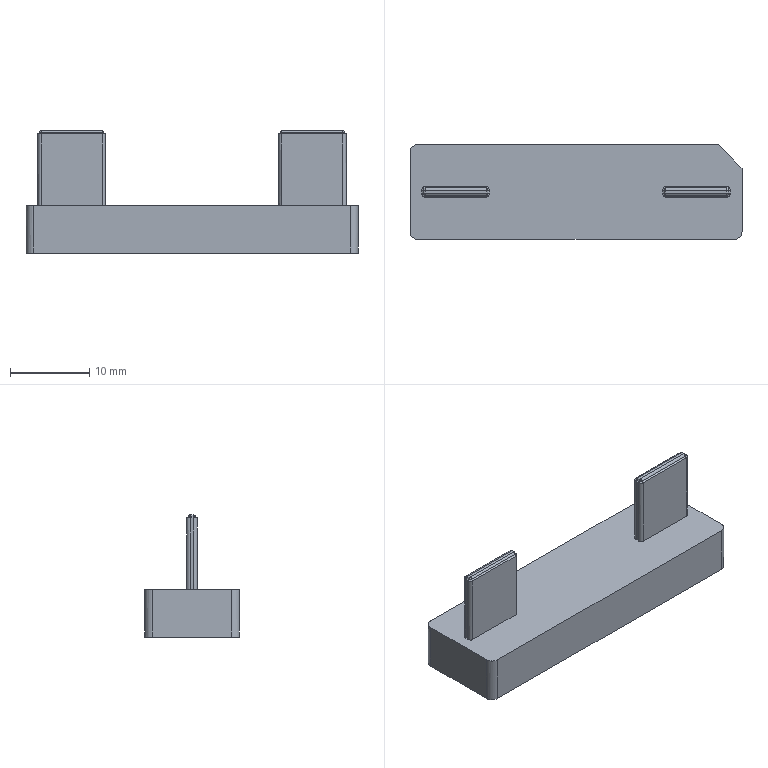NC program | PowerMill | posted with a generic post | part box 42 x 12 x 15.447 mm
Lines 5063 to 6058 of 88764:
N5160 M6
N5161 S18000 M03
N5162 G00 G90 X0.0 Y0.0
N5163 G43 Z9.7972 H2
N5164
N5165 G05 P10000 R4
N5166 X-16.8455 Y3.4637
N5167 Z0.7877
N5168 G01 Z-0.4123 F3600.0
N5169 X-16.8553 Y3.444 F6000.0
N5170 G03 X-16.7667 Y3.1783 I0.1771 J-0.0885
N5171 G01 X-15.3737 Y2.4822
N5172 X-11.7133 Y2.4829
N5173 X-11.2252 Y2.4763
N5174 X-10.7372 Y2.3846
N5175 X-10.2969 Y2.1962
N5176 X-9.7611 Y1.7673
N5177 X-9.3902 Y1.2201
N5178 X-9.2227 Y0.7321
N5179 X-9.1642 Y0.244
N5180 X-9.1662 Y-0.244
N5181 X-9.2316 Y-0.7321
N5182 X-9.4063 Y-1.2201
N5183 X-9.7365 Y-1.7082
N5184 X-10.2491 Y-2.1361
N5185 X-10.3552 Y-2.1962
N5186 X-10.7372 Y-2.3486
N5187 X-11.2252 Y-2.442
N5188 X-11.7133 Y-2.4487
N5189 X-19.0341 Y-2.4496
N5190 X-19.5221 Y-2.4047
N5191 X-20.0102 Y-2.2512
N5192 X-20.4982 Y-1.9437
N5193 X-20.7437 Y-1.7082
N5194 X-20.9863 Y-1.3814
N5195 X-21.0744 Y-1.2201
N5196 X-21.2494 Y-0.7321
N5197 X-21.3146 Y-0.244
N5198 X-21.3168 Y0.244
N5199 X-21.257 Y0.7321
N5200 X-21.0904 Y1.2201
N5201 X-20.9863 Y1.4141
N5202 X-20.7731 Y1.7082
N5203 X-20.4982 Y1.9737
N5204 X-20.184 Y2.1962
N5205 X-20.0102 Y2.2853
N5206 X-19.5221 Y2.4377
N5207 X-19.0341 Y2.4814
N5208 X-15.3737 Y2.4822
N5209 X-16.8055 Y3.6441 Z-0.6116
N5210 X-16.8154 Y3.6245
N5211 G03 X-16.7268 Y3.3588 I0.1771 J-0.0886
N5212 G01 X-15.3737 Y2.6822
N5213 X-11.7133
N5214 X-11.2252 Y2.6769
N5215 X-10.7372 Y2.5943
N5216 X-10.2491 Y2.3983
N5217 X-9.9368 Y2.1962
N5218 X-9.7611 Y2.0517
N5219 X-9.4529 Y1.7082
N5220 X-9.273 Y1.4244
N5221 X-9.1745 Y1.2201
N5222 X-9.0244 Y0.7321
N5223 X-8.9752 Y0.244
N5224 X-8.9755 Y-0.244
N5225 X-9.0306 Y-0.7321
N5226 X-9.1881 Y-1.2201
N5227 X-9.4766 Y-1.7082
N5228 X-9.7611 Y-2.0182
N5229 X-9.9783 Y-2.1962
N5230 X-10.2491 Y-2.3659
N5231 X-10.7372 Y-2.5618
N5232 X-11.2252 Y-2.6441
N5233 X-11.7133 Y-2.65
N5234 X-19.0341
N5235 X-19.5221 Y-2.6099
N5236 X-20.0102 Y-2.4692
N5237 X-20.4982 Y-2.1971
N5238 X-20.9863 Y-1.7303
N5239 X-21.2917 Y-1.2201
N5240 X-21.4492 Y-0.7321
N5241 X-21.5045 Y-0.244
N5242 X-21.5048 Y0.244
N5243 X-21.4743 Y0.6236
N5244 X-21.3056 Y1.2201
N5245 X-21.0273 Y1.7082
N5246 X-20.545 Y2.1962
N5247 X-20.0102 Y2.5013
N5248 X-19.5221 Y2.6441
N5249 X-19.0341 Y2.6822
N5250 X-15.3737
N5251 X-16.8055 Y3.6441 Z-0.8109
N5252 X-16.8154 Y3.6245
N5253 G03 X-16.7268 Y3.3588 I0.1771 J-0.0886
N5254 G01 X-15.3737 Y2.6822
N5255 X-11.7133
N5256 X-11.2252 Y2.6769
N5257 X-10.7372 Y2.5943
N5258 X-10.2491 Y2.3983
N5259 X-9.9368 Y2.1962
N5260 X-9.7611 Y2.0517
N5261 X-9.4529 Y1.7082
N5262 X-9.273 Y1.4244
N5263 X-9.1745 Y1.2201
N5264 X-9.0244 Y0.7321
N5265 X-8.9752 Y0.244
N5266 X-8.9755 Y-0.244
N5267 X-9.0306 Y-0.7321
N5268 X-9.1881 Y-1.2201
N5269 X-9.4766 Y-1.7082
N5270 X-9.7611 Y-2.0182
N5271 X-9.9783 Y-2.1962
N5272 X-10.2491 Y-2.3659
N5273 X-10.7372 Y-2.5618
N5274 X-11.2252 Y-2.6441
N5275 X-11.7133 Y-2.65
N5276 X-19.0341
N5277 X-19.5221 Y-2.6099
N5278 X-20.0102 Y-2.4692
N5279 X-20.4982 Y-2.1971
N5280 X-20.9863 Y-1.7303
N5281 X-21.2917 Y-1.2201
N5282 X-21.4492 Y-0.7321
N5283 X-21.5045 Y-0.244
N5284 X-21.5048 Y0.244
N5285 X-21.4743 Y0.6236
N5286 X-21.3056 Y1.2201
N5287 X-21.0273 Y1.7082
N5288 X-20.545 Y2.1962
N5289 X-20.0102 Y2.5013
N5290 X-19.5221 Y2.6441
N5291 X-19.0341 Y2.6822
N5292 X-15.3737
N5293 X-16.8055 Y3.6441 Z-1.0102
N5294 X-16.8154 Y3.6245
N5295 G03 X-16.7268 Y3.3588 I0.1771 J-0.0886
N5296 G01 X-15.3737 Y2.6822
N5297 X-11.7133
N5298 X-11.2252 Y2.6769
N5299 X-10.7372 Y2.5943
N5300 X-10.2491 Y2.3983
N5301 X-9.9368 Y2.1962
N5302 X-9.7611 Y2.0517
N5303 X-9.4529 Y1.7082
N5304 X-9.273 Y1.4245
N5305 X-9.1745 Y1.2201
N5306 X-9.0244 Y0.7321
N5307 X-8.9752 Y0.244
N5308 X-8.9755 Y-0.244
N5309 X-9.0306 Y-0.7321
N5310 X-9.1881 Y-1.2201
N5311 X-9.4766 Y-1.7082
N5312 X-9.7611 Y-2.0182
N5313 X-9.9783 Y-2.1962
N5314 X-10.2491 Y-2.3659
N5315 X-10.7372 Y-2.5618
N5316 X-11.2252 Y-2.6441
N5317 X-11.7133 Y-2.65
N5318 X-19.0341
N5319 X-19.5221 Y-2.61
N5320 X-20.0102 Y-2.4692
N5321 X-20.4982 Y-2.1971
N5322 X-20.9863 Y-1.7303
N5323 X-21.2918 Y-1.2201
N5324 X-21.4492 Y-0.7321
N5325 X-21.5045 Y-0.244
N5326 X-21.5048 Y0.244
N5327 X-21.4743 Y0.6236
N5328 X-21.3056 Y1.2201
N5329 X-21.0273 Y1.7082
N5330 X-20.545 Y2.1962
N5331 X-20.0102 Y2.5013
N5332 X-19.5221 Y2.6441
N5333 X-19.0341 Y2.6822
N5334 X-15.3737
N5335 X-16.8055 Y3.6441 Z-1.2095
N5336 X-16.8154 Y3.6245
N5337 G03 X-16.7268 Y3.3588 I0.1771 J-0.0886
N5338 G01 X-15.3737 Y2.6822
N5339 X-11.7133
N5340 X-11.2252 Y2.6769
N5341 X-10.7372 Y2.5943
N5342 X-10.2491 Y2.3983
N5343 X-9.9368 Y2.1962
N5344 X-9.7611 Y2.0517
N5345 X-9.4529 Y1.7082
N5346 X-9.273 Y1.4245
N5347 X-9.1745 Y1.2201
N5348 X-9.0244 Y0.7321
N5349 X-8.9752 Y0.244
N5350 X-8.9755 Y-0.244
N5351 X-9.0306 Y-0.7321
N5352 X-9.1881 Y-1.2201
N5353 X-9.4766 Y-1.7082
N5354 X-9.7611 Y-2.0182
N5355 X-9.9783 Y-2.1962
N5356 X-10.2491 Y-2.3659
N5357 X-10.7372 Y-2.5618
N5358 X-11.2252 Y-2.6441
N5359 X-11.7133 Y-2.65
N5360 X-19.0341
N5361 X-19.5221 Y-2.61
N5362 X-20.0102 Y-2.4692
N5363 X-20.4982 Y-2.1971
N5364 X-20.9863 Y-1.7303
N5365 X-21.2918 Y-1.2201
N5366 X-21.4492 Y-0.7321
N5367 X-21.5045 Y-0.244
N5368 X-21.5048 Y0.244
N5369 X-21.4743 Y0.6236
N5370 X-21.3056 Y1.2201
N5371 X-21.0273 Y1.7082
N5372 X-20.545 Y2.1962
N5373 X-20.0102 Y2.5013
N5374 X-19.5221 Y2.6441
N5375 X-19.0341 Y2.6822
N5376 X-15.3737
N5377 X-16.8055 Y3.6441 Z-1.4088
N5378 X-16.8154 Y3.6245
N5379 G03 X-16.7268 Y3.3588 I0.1771 J-0.0886
N5380 G01 X-15.3737 Y2.6822
N5381 X-11.7133
N5382 X-11.2252 Y2.6769
N5383 X-10.7372 Y2.5943
N5384 X-10.2491 Y2.3983
N5385 X-9.9368 Y2.1962
N5386 X-9.7611 Y2.0517
N5387 X-9.4529 Y1.7082
N5388 X-9.273 Y1.4245
N5389 X-9.1745 Y1.2201
N5390 X-9.0244 Y0.7321
N5391 X-8.9752 Y0.244
N5392 X-8.9755 Y-0.244
N5393 X-9.0306 Y-0.7321
N5394 X-9.1881 Y-1.2201
N5395 X-9.4766 Y-1.7082
N5396 X-9.7611 Y-2.0182
N5397 X-9.9783 Y-2.1962
N5398 X-10.2491 Y-2.3659
N5399 X-10.7372 Y-2.5618
N5400 X-11.2252 Y-2.6441
N5401 X-11.7133 Y-2.65
N5402 X-19.0341
N5403 X-19.5221 Y-2.61
N5404 X-20.0102 Y-2.4692
N5405 X-20.4982 Y-2.1971
N5406 X-20.9863 Y-1.7303
N5407 X-21.2918 Y-1.2201
N5408 X-21.4492 Y-0.7321
N5409 X-21.5045 Y-0.244
N5410 X-21.5048 Y0.244
N5411 X-21.4743 Y0.6236
N5412 X-21.3056 Y1.2201
N5413 X-21.0273 Y1.7082
N5414 X-20.545 Y2.1962
N5415 X-20.0102 Y2.5014
N5416 X-19.5221 Y2.6441
N5417 X-19.0341 Y2.6822
N5418 X-15.3737
N5419 X-16.8055 Y3.6441 Z-1.6081
N5420 X-16.8154 Y3.6245
N5421 G03 X-16.7268 Y3.3588 I0.1771 J-0.0886
N5422 G01 X-15.3737 Y2.6822
N5423 X-11.7133
N5424 X-11.2252 Y2.6769
N5425 X-10.7372 Y2.5943
N5426 X-10.2491 Y2.3983
N5427 X-9.9368 Y2.1962
N5428 X-9.7611 Y2.0517
N5429 X-9.4529 Y1.7082
N5430 X-9.273 Y1.4245
N5431 X-9.1745 Y1.2201
N5432 X-9.0244 Y0.7321
N5433 X-8.9752 Y0.244
N5434 X-8.9755 Y-0.244
N5435 X-9.0306 Y-0.7321
N5436 X-9.1881 Y-1.2201
N5437 X-9.4766 Y-1.7082
N5438 X-9.7611 Y-2.0182
N5439 X-9.9783 Y-2.1962
N5440 X-10.2491 Y-2.3659
N5441 X-10.7372 Y-2.5618
N5442 X-11.2252 Y-2.6441
N5443 X-11.7133 Y-2.65
N5444 X-19.0341
N5445 X-19.5221 Y-2.61
N5446 X-20.0102 Y-2.4692
N5447 X-20.4982 Y-2.1971
N5448 X-20.9863 Y-1.7304
N5449 X-21.2918 Y-1.2201
N5450 X-21.4492 Y-0.7321
N5451 X-21.5046 Y-0.244
N5452 X-21.5048 Y0.244
N5453 X-21.4743 Y0.6237
N5454 X-21.3056 Y1.2201
N5455 X-21.0273 Y1.7082
N5456 X-20.545 Y2.1962
N5457 X-20.0102 Y2.5014
N5458 X-19.5221 Y2.6441
N5459 X-19.0341 Y2.6822
N5460 X-15.3737
N5461 X-16.8055 Y3.6441 Z-1.8074
N5462 X-16.8154 Y3.6245
N5463 G03 X-16.7268 Y3.3588 I0.1771 J-0.0886
N5464 G01 X-15.3737 Y2.6822
N5465 X-11.7133
N5466 X-11.2252 Y2.6769
N5467 X-10.7372 Y2.5943
N5468 X-10.2491 Y2.3983
N5469 X-9.9368 Y2.1962
N5470 X-9.7611 Y2.0517
N5471 X-9.4529 Y1.7082
N5472 X-9.273 Y1.4245
N5473 X-9.1745 Y1.2201
N5474 X-9.0244 Y0.7321
N5475 X-8.9752 Y0.244
N5476 X-8.9755 Y-0.244
N5477 X-9.0306 Y-0.7321
N5478 X-9.1881 Y-1.2201
N5479 X-9.4766 Y-1.7082
N5480 X-9.7611 Y-2.0182
N5481 X-9.9783 Y-2.1962
N5482 X-10.2491 Y-2.3659
N5483 X-10.7372 Y-2.5618
N5484 X-11.2252 Y-2.6441
N5485 X-11.7133 Y-2.65
N5486 X-19.0341
N5487 X-19.5221 Y-2.61
N5488 X-20.0102 Y-2.4692
N5489 X-20.4982 Y-2.1971
N5490 X-20.9863 Y-1.7304
N5491 X-21.2918 Y-1.2201
N5492 X-21.4492 Y-0.7321
N5493 X-21.5046 Y-0.244
N5494 X-21.5048 Y0.244
N5495 X-21.4743 Y0.6237
N5496 X-21.3056 Y1.2201
N5497 X-21.0273 Y1.7082
N5498 X-20.545 Y2.1962
N5499 X-20.0102 Y2.5014
N5500 X-19.5221 Y2.6441
N5501 X-19.0341 Y2.6822
N5502 X-15.3737
N5503 X-16.8055 Y3.6441 Z-2.0067
N5504 X-16.8154 Y3.6245
N5505 G03 X-16.7268 Y3.3588 I0.1771 J-0.0886
N5506 G01 X-15.3737 Y2.6822
N5507 X-11.7133
N5508 X-11.2252 Y2.677
N5509 X-10.7372 Y2.5943
N5510 X-10.2491 Y2.3983
N5511 X-9.9368 Y2.1962
N5512 X-9.7611 Y2.0517
N5513 X-9.4529 Y1.7082
N5514 X-9.273 Y1.4245
N5515 X-9.1745 Y1.2201
N5516 X-9.0244 Y0.7321
N5517 X-8.9752 Y0.244
N5518 X-8.9755 Y-0.244
N5519 X-9.0306 Y-0.7321
N5520 X-9.1881 Y-1.2201
N5521 X-9.4766 Y-1.7082
N5522 X-9.7611 Y-2.0182
N5523 X-9.9783 Y-2.1962
N5524 X-10.2491 Y-2.3659
N5525 X-10.7372 Y-2.5618
N5526 X-11.2252 Y-2.6441
N5527 X-11.7133 Y-2.65
N5528 X-19.0341
N5529 X-19.5221 Y-2.61
N5530 X-20.0102 Y-2.4692
N5531 X-20.4982 Y-2.1971
N5532 X-20.9863 Y-1.7304
N5533 X-21.2918 Y-1.2201
N5534 X-21.4492 Y-0.7321
N5535 X-21.5046 Y-0.244
N5536 X-21.5048 Y0.244
N5537 X-21.4743 Y0.6237
N5538 X-21.3056 Y1.2201
N5539 X-21.0273 Y1.7082
N5540 X-20.545 Y2.1962
N5541 X-20.0102 Y2.5014
N5542 X-19.5221 Y2.6441
N5543 X-19.0341 Y2.6822
N5544 X-15.3737
N5545 X-16.8055 Y3.6441 Z-2.206
N5546 X-16.8154 Y3.6245
N5547 G03 X-16.7268 Y3.3588 I0.1771 J-0.0886
N5548 G01 X-15.3737 Y2.6822
N5549 X-11.7133
N5550 X-11.2252 Y2.677
N5551 X-10.7372 Y2.5943
N5552 X-10.2491 Y2.3983
N5553 X-9.9368 Y2.1962
N5554 X-9.7611 Y2.0517
N5555 X-9.4529 Y1.7082
N5556 X-9.273 Y1.4245
N5557 X-9.1745 Y1.2201
N5558 X-9.0244 Y0.7321
N5559 X-8.9752 Y0.244
N5560 X-8.9755 Y-0.244
N5561 X-9.0306 Y-0.7321
N5562 X-9.1881 Y-1.2201
N5563 X-9.4766 Y-1.7082
N5564 X-9.7611 Y-2.0182
N5565 X-9.9783 Y-2.1962
N5566 X-10.2491 Y-2.3659
N5567 X-10.7372 Y-2.5618
N5568 X-11.2252 Y-2.6441
N5569 X-11.7133 Y-2.6501
N5570 X-19.0341
N5571 X-19.5221 Y-2.61
N5572 X-20.0102 Y-2.4692
N5573 X-20.4982 Y-2.1971
N5574 X-20.9863 Y-1.7304
N5575 X-21.2918 Y-1.2201
N5576 X-21.4492 Y-0.7321
N5577 X-21.5046 Y-0.244
N5578 X-21.5048 Y0.244
N5579 X-21.4743 Y0.6237
N5580 X-21.3056 Y1.2201
N5581 X-21.0273 Y1.7082
N5582 X-20.545 Y2.1962
N5583 X-20.0102 Y2.5014
N5584 X-19.5221 Y2.6441
N5585 X-19.0341 Y2.6822
N5586 X-15.3737
N5587 X-16.8055 Y3.6441 Z-2.4053
N5588 X-16.8154 Y3.6245
N5589 G03 X-16.7268 Y3.3588 I0.1771 J-0.0886
N5590 G01 X-15.3737 Y2.6823
N5591 X-11.7133
N5592 X-11.2252 Y2.677
N5593 X-10.7372 Y2.5943
N5594 X-10.2491 Y2.3983
N5595 X-9.9368 Y2.1962
N5596 X-9.7611 Y2.0517
N5597 X-9.4529 Y1.7082
N5598 X-9.273 Y1.4245
N5599 X-9.1745 Y1.2201
N5600 X-9.0244 Y0.7321
N5601 X-8.9752 Y0.244
N5602 X-8.9755 Y-0.244
N5603 X-9.0306 Y-0.7321
N5604 X-9.1881 Y-1.2201
N5605 X-9.4766 Y-1.7082
N5606 X-9.7611 Y-2.0182
N5607 X-9.9783 Y-2.1962
N5608 X-10.2491 Y-2.3659
N5609 X-10.7372 Y-2.5618
N5610 X-11.2252 Y-2.6441
N5611 X-11.7133 Y-2.6501
N5612 X-19.0341
N5613 X-19.5221 Y-2.61
N5614 X-20.0102 Y-2.4692
N5615 X-20.4982 Y-2.1971
N5616 X-20.9863 Y-1.7304
N5617 X-21.2918 Y-1.2201
N5618 X-21.4492 Y-0.7321
N5619 X-21.5046 Y-0.244
N5620 X-21.5048 Y0.244
N5621 X-21.4743 Y0.6237
N5622 X-21.3056 Y1.2201
N5623 X-21.0273 Y1.7082
N5624 X-20.545 Y2.1962
N5625 X-20.0102 Y2.5014
N5626 X-19.5221 Y2.6441
N5627 X-19.0341 Y2.6823
N5628 X-15.3737
N5629 X-16.8055 Y3.6442 Z-2.6046
N5630 X-16.8154 Y3.6245
N5631 G03 X-16.7268 Y3.3588 I0.1771 J-0.0886
N5632 G01 X-15.3737 Y2.6823
N5633 X-11.7133
N5634 X-11.2252 Y2.677
N5635 X-10.7372 Y2.5943
N5636 X-10.2491 Y2.3983
N5637 X-9.9368 Y2.1962
N5638 X-9.7611 Y2.0517
N5639 X-9.4529 Y1.7082
N5640 X-9.273 Y1.4245
N5641 X-9.1745 Y1.2201
N5642 X-9.0244 Y0.7321
N5643 X-8.9752 Y0.244
N5644 X-8.9755 Y-0.244
N5645 X-9.0306 Y-0.7321
N5646 X-9.1881 Y-1.2201
N5647 X-9.4766 Y-1.7082
N5648 X-9.7611 Y-2.0182
N5649 X-9.9783 Y-2.1962
N5650 X-10.2491 Y-2.3659
N5651 X-10.7372 Y-2.5618
N5652 X-11.2252 Y-2.6441
N5653 X-11.7133 Y-2.6501
N5654 X-19.0341
N5655 X-19.5221 Y-2.61
N5656 X-20.0102 Y-2.4692
N5657 X-20.4982 Y-2.1971
N5658 X-20.9863 Y-1.7304
N5659 X-21.2918 Y-1.2201
N5660 X-21.4492 Y-0.7321
N5661 X-21.5046 Y-0.244
N5662 X-21.5048 Y0.244
N5663 X-21.4743 Y0.6237
N5664 X-21.3056 Y1.2201
N5665 X-21.0273 Y1.7082
N5666 X-20.545 Y2.1962
N5667 X-20.0102 Y2.5014
N5668 X-19.5221 Y2.6441
N5669 X-19.0341 Y2.6823
N5670 X-15.3737
N5671 X-16.8055 Y3.6442 Z-2.8039
N5672 X-16.8154 Y3.6245
N5673 G03 X-16.7268 Y3.3588 I0.1771 J-0.0886
N5674 G01 X-15.3737 Y2.6823
N5675 X-11.7133
N5676 X-11.2252 Y2.677
N5677 X-10.7372 Y2.5943
N5678 X-10.2491 Y2.3983
N5679 X-9.9368 Y2.1962
N5680 X-9.7611 Y2.0517
N5681 X-9.4529 Y1.7082
N5682 X-9.273 Y1.4245
N5683 X-9.1745 Y1.2201
N5684 X-9.0244 Y0.7321
N5685 X-8.9752 Y0.244
N5686 X-8.9755 Y-0.244
N5687 X-9.0306 Y-0.7321
N5688 X-9.1881 Y-1.2201
N5689 X-9.4766 Y-1.7082
N5690 X-9.7611 Y-2.0182
N5691 X-9.9783 Y-2.1962
N5692 X-10.2491 Y-2.3659
N5693 X-10.7372 Y-2.5618
N5694 X-11.2252 Y-2.6441
N5695 X-11.7133 Y-2.6501
N5696 X-19.0341
N5697 X-19.5221 Y-2.61
N5698 X-20.0102 Y-2.4692
N5699 X-20.4982 Y-2.1971
N5700 X-20.9863 Y-1.7304
N5701 X-21.2918 Y-1.2201
N5702 X-21.4492 Y-0.7321
N5703 X-21.5046 Y-0.244
N5704 X-21.5048 Y0.244
N5705 X-21.4743 Y0.6237
N5706 X-21.3056 Y1.2201
N5707 X-21.0273 Y1.7082
N5708 X-20.545 Y2.1962
N5709 X-20.0102 Y2.5014
N5710 X-19.5221 Y2.6441
N5711 X-19.0341 Y2.6823
N5712 X-15.3737
N5713 X-16.8055 Y3.6442 Z-3.0032
N5714 X-16.8154 Y3.6245
N5715 G03 X-16.7268 Y3.3588 I0.1771 J-0.0886
N5716 G01 X-15.3737 Y2.6823
N5717 X-11.7133
N5718 X-11.2252 Y2.677
N5719 X-10.7372 Y2.5943
N5720 X-10.2491 Y2.3983
N5721 X-9.9368 Y2.1962
N5722 X-9.7611 Y2.0517
N5723 X-9.4529 Y1.7082
N5724 X-9.273 Y1.4245
N5725 X-9.1745 Y1.2201
N5726 X-9.0243 Y0.7321
N5727 X-8.9752 Y0.244
N5728 X-8.9755 Y-0.244
N5729 X-9.0306 Y-0.7321
N5730 X-9.1881 Y-1.2201
N5731 X-9.4766 Y-1.7082
N5732 X-9.7611 Y-2.0182
N5733 X-9.9783 Y-2.1962
N5734 X-10.2491 Y-2.3659
N5735 X-10.7372 Y-2.5618
N5736 X-11.2252 Y-2.6441
N5737 X-11.7133 Y-2.6501
N5738 X-19.0341
N5739 X-19.5221 Y-2.61
N5740 X-20.0102 Y-2.4692
N5741 X-20.4982 Y-2.1971
N5742 X-20.9863 Y-1.7304
N5743 X-21.2918 Y-1.2201
N5744 X-21.4492 Y-0.7321
N5745 X-21.5046 Y-0.244
N5746 X-21.5048 Y0.244
N5747 X-21.4743 Y0.6237
N5748 X-21.3056 Y1.2201
N5749 X-21.0273 Y1.7082
N5750 X-20.545 Y2.1962
N5751 X-20.0102 Y2.5014
N5752 X-19.5221 Y2.6441
N5753 X-19.0341 Y2.6823
N5754 X-15.3737
N5755 X-16.8055 Y3.6442 Z-3.2025
N5756 X-16.8154 Y3.6245
N5757 G03 X-16.7268 Y3.3588 I0.1771 J-0.0886
N5758 G01 X-15.3737 Y2.6823
N5759 X-11.7133
N5760 X-11.2252 Y2.677
N5761 X-10.7372 Y2.5943
N5762 X-10.2491 Y2.3983
N5763 X-9.9368 Y2.1962
N5764 X-9.7611 Y2.0517
N5765 X-9.4529 Y1.7082
N5766 X-9.273 Y1.4245
N5767 X-9.1745 Y1.2201
N5768 X-9.0243 Y0.7321
N5769 X-8.9752 Y0.244
N5770 X-8.9755 Y-0.244
N5771 X-9.0306 Y-0.7321
N5772 X-9.1881 Y-1.2201
N5773 X-9.4766 Y-1.7082
N5774 X-9.7611 Y-2.0182
N5775 X-9.9783 Y-2.1962
N5776 X-10.2491 Y-2.3659
N5777 X-10.7372 Y-2.5618
N5778 X-11.2252 Y-2.6441
N5779 X-11.7133 Y-2.6501
N5780 X-19.0341
N5781 X-19.5221 Y-2.61
N5782 X-20.0102 Y-2.4692
N5783 X-20.4982 Y-2.1971
N5784 X-20.9863 Y-1.7304
N5785 X-21.2918 Y-1.2201
N5786 X-21.4492 Y-0.7321
N5787 X-21.5046 Y-0.244
N5788 X-21.5048 Y0.244
N5789 X-21.4743 Y0.6237
N5790 X-21.3056 Y1.2201
N5791 X-21.0273 Y1.7082
N5792 X-20.545 Y2.1962
N5793 X-20.0102 Y2.5014
N5794 X-19.5221 Y2.6441
N5795 X-19.0341 Y2.6823
N5796 X-15.3737
N5797 X-16.8055 Y3.6442 Z-3.4018
N5798 X-16.8154 Y3.6245
N5799 G03 X-16.7268 Y3.3588 I0.1771 J-0.0886
N5800 G01 X-15.3737 Y2.6823
N5801 X-11.7133
N5802 X-11.2252 Y2.677
N5803 X-10.7372 Y2.5943
N5804 X-10.2491 Y2.3983
N5805 X-9.9368 Y2.1962
N5806 X-9.7611 Y2.0517
N5807 X-9.4529 Y1.7082
N5808 X-9.273 Y1.4245
N5809 X-9.1745 Y1.2201
N5810 X-9.0243 Y0.7321
N5811 X-8.9752 Y0.244
N5812 X-8.9755 Y-0.244
N5813 X-9.0306 Y-0.7321
N5814 X-9.1881 Y-1.2201
N5815 X-9.4766 Y-1.7082
N5816 X-9.7611 Y-2.0182
N5817 X-9.9783 Y-2.1962
N5818 X-10.2491 Y-2.3659
N5819 X-10.7372 Y-2.5618
N5820 X-11.2252 Y-2.6441
N5821 X-11.7133 Y-2.6501
N5822 X-19.0341
N5823 X-19.5221 Y-2.61
N5824 X-20.0102 Y-2.4692
N5825 X-20.4982 Y-2.1971
N5826 X-20.9863 Y-1.7304
N5827 X-21.2918 Y-1.2201
N5828 X-21.4492 Y-0.7321
N5829 X-21.5046 Y-0.244
N5830 X-21.5048 Y0.244
N5831 X-21.4743 Y0.6237
N5832 X-21.3056 Y1.2201
N5833 X-21.0273 Y1.7082
N5834 X-20.545 Y2.1962
N5835 X-20.0102 Y2.5014
N5836 X-19.5221 Y2.6441
N5837 X-19.0341 Y2.6823
N5838 X-15.3737
N5839 X-16.8055 Y3.6442 Z-3.6011
N5840 X-16.8154 Y3.6245
N5841 G03 X-16.7268 Y3.3588 I0.1771 J-0.0886
N5842 G01 X-15.3737 Y2.6823
N5843 X-11.7133
N5844 X-11.2252 Y2.677
N5845 X-10.7372 Y2.5943
N5846 X-10.2491 Y2.3983
N5847 X-9.9368 Y2.1962
N5848 X-9.7611 Y2.0517
N5849 X-9.4529 Y1.7082
N5850 X-9.273 Y1.4245
N5851 X-9.1745 Y1.2201
N5852 X-9.0243 Y0.7321
N5853 X-8.9752 Y0.244
N5854 X-8.9755 Y-0.244
N5855 X-9.0306 Y-0.7321
N5856 X-9.1881 Y-1.2201
N5857 X-9.4766 Y-1.7082
N5858 X-9.7611 Y-2.0182
N5859 X-9.9783 Y-2.1962
N5860 X-10.2491 Y-2.3659
N5861 X-10.7372 Y-2.5618
N5862 X-11.2252 Y-2.6441
N5863 X-11.7133 Y-2.6501
N5864 X-19.0341
N5865 X-19.5221 Y-2.61
N5866 X-20.0102 Y-2.4692
N5867 X-20.4982 Y-2.1971
N5868 X-20.9863 Y-1.7304
N5869 X-21.2918 Y-1.2201
N5870 X-21.4492 Y-0.7321
N5871 X-21.5046 Y-0.244
N5872 X-21.5048 Y0.244
N5873 X-21.4743 Y0.6237
N5874 X-21.3056 Y1.2201
N5875 X-21.0273 Y1.7082
N5876 X-20.545 Y2.1962
N5877 X-20.0102 Y2.5014
N5878 X-19.5221 Y2.6441
N5879 X-19.0341 Y2.6823
N5880 X-15.3737
N5881 X-16.8055 Y3.6442 Z-3.8004
N5882 X-16.8154 Y3.6245
N5883 G03 X-16.7268 Y3.3588 I0.1771 J-0.0886
N5884 G01 X-15.3737 Y2.6823
N5885 X-11.7133
N5886 X-11.2252 Y2.677
N5887 X-10.7372 Y2.5943
N5888 X-10.2491 Y2.3983
N5889 X-9.9368 Y2.1962
N5890 X-9.7611 Y2.0517
N5891 X-9.4529 Y1.7082
N5892 X-9.273 Y1.4245
N5893 X-9.1745 Y1.2201
N5894 X-9.0243 Y0.7321
N5895 X-8.9752 Y0.244
N5896 X-8.9755 Y-0.244
N5897 X-9.0306 Y-0.7321
N5898 X-9.1881 Y-1.2201
N5899 X-9.4766 Y-1.7082
N5900 X-9.7611 Y-2.0182
N5901 X-9.9783 Y-2.1962
N5902 X-10.2491 Y-2.3659
N5903 X-10.7372 Y-2.5618
N5904 X-11.2252 Y-2.6441
N5905 X-11.7133 Y-2.6501
N5906 X-19.0341
N5907 X-19.5221 Y-2.61
N5908 X-20.0102 Y-2.4692
N5909 X-20.4982 Y-2.1971
N5910 X-20.9863 Y-1.7304
N5911 X-21.2918 Y-1.2201
N5912 X-21.4492 Y-0.7321
N5913 X-21.5046 Y-0.244
N5914 X-21.5048 Y0.244
N5915 X-21.4743 Y0.6237
N5916 X-21.3056 Y1.2201
N5917 X-21.0273 Y1.7082
N5918 X-20.545 Y2.1962
N5919 X-20.0102 Y2.5014
N5920 X-19.5221 Y2.6441
N5921 X-19.0341 Y2.6823
N5922 X-15.3737
N5923 X-16.8055 Y3.6442 Z-3.9997
N5924 X-16.8153 Y3.6245
N5925 G03 X-16.7268 Y3.3588 I0.177 J-0.0886
N5926 G01 X-15.3737 Y2.6823
N5927 X-11.7133
N5928 X-11.2252 Y2.677
N5929 X-10.7372 Y2.5943
N5930 X-10.2491 Y2.3983
N5931 X-9.9368 Y2.1962
N5932 X-9.7611 Y2.0517
N5933 X-9.4529 Y1.7082
N5934 X-9.273 Y1.4245
N5935 X-9.1745 Y1.2201
N5936 X-9.0243 Y0.7321
N5937 X-8.9752 Y0.244
N5938 X-8.9755 Y-0.244
N5939 X-9.0306 Y-0.7321
N5940 X-9.1881 Y-1.2201
N5941 X-9.4766 Y-1.7082
N5942 X-9.7611 Y-2.0182
N5943 X-9.9783 Y-2.1962
N5944 X-10.2491 Y-2.3659
N5945 X-10.7372 Y-2.5618
N5946 X-11.2252 Y-2.6441
N5947 X-11.7133 Y-2.6501
N5948 X-19.0341
N5949 X-19.5221 Y-2.61
N5950 X-20.0102 Y-2.4692
N5951 X-20.4982 Y-2.1971
N5952 X-20.9863 Y-1.7304
N5953 X-21.2918 Y-1.2201
N5954 X-21.4493 Y-0.7321
N5955 X-21.5046 Y-0.244
N5956 X-21.5048 Y0.244
N5957 X-21.4743 Y0.6237
N5958 X-21.3056 Y1.2201
N5959 X-21.0273 Y1.7082
N5960 X-20.545 Y2.1962
N5961 X-20.0102 Y2.5014
N5962 X-19.5221 Y2.6441
N5963 X-19.0341 Y2.6823
N5964 X-15.3737
N5965 X-16.8055 Y3.6442 Z-4.1989
N5966 X-16.8153 Y3.6245
N5967 G03 X-16.7268 Y3.3588 I0.177 J-0.0886
N5968 G01 X-15.3737 Y2.6823
N5969 X-11.7133
N5970 X-11.2252 Y2.677
N5971 X-10.7372 Y2.5943
N5972 X-10.2491 Y2.3983
N5973 X-9.9368 Y2.1962
N5974 X-9.7611 Y2.0517
N5975 X-9.4529 Y1.7082
N5976 X-9.273 Y1.4245
N5977 X-9.1745 Y1.2201
N5978 X-9.0243 Y0.7321
N5979 X-8.9752 Y0.244
N5980 X-8.9755 Y-0.244
N5981 X-9.0306 Y-0.7321
N5982 X-9.1881 Y-1.2201
N5983 X-9.4766 Y-1.7082
N5984 X-9.7611 Y-2.0182
N5985 X-9.9783 Y-2.1962
N5986 X-10.2491 Y-2.3659
N5987 X-10.7372 Y-2.5618
N5988 X-11.2252 Y-2.6441
N5989 X-11.7133 Y-2.6501
N5990 X-19.0341
N5991 X-19.5221 Y-2.61
N5992 X-20.0102 Y-2.4692
N5993 X-20.4982 Y-2.1971
N5994 X-20.9863 Y-1.7304
N5995 X-21.2918 Y-1.2201
N5996 X-21.4493 Y-0.7321
N5997 X-21.5046 Y-0.244
N5998 X-21.5048 Y0.244
N5999 X-21.4743 Y0.6237
N6000 X-21.3056 Y1.2201
N6001 X-21.0273 Y1.7082
N6002 X-20.545 Y2.1962
N6003 X-20.0102 Y2.5014
N6004 X-19.5221 Y2.6441
N6005 X-19.0341 Y2.6823
N6006 X-15.3737
N6007 X-16.8055 Y3.6442 Z-4.3983
N6008 X-16.8153 Y3.6245
N6009 G03 X-16.7268 Y3.3588 I0.1771 J-0.0886
N6010 G01 X-15.3737 Y2.6823
N6011 X-11.7133
N6012 X-11.2252 Y2.677
N6013 X-10.7372 Y2.5943
N6014 X-10.2491 Y2.3983
N6015 X-9.9368 Y2.1962
N6016 X-9.7611 Y2.0517
N6017 X-9.4529 Y1.7082
N6018 X-9.273 Y1.4245
N6019 X-9.1745 Y1.2201
N6020 X-9.0243 Y0.7321
N6021 X-8.9752 Y0.244
N6022 X-8.9755 Y-0.244
N6023 X-9.0306 Y-0.7321
N6024 X-9.1881 Y-1.2201
N6025 X-9.4766 Y-1.7082
N6026 X-9.7611 Y-2.0182
N6027 X-9.9783 Y-2.1962
N6028 X-10.2491 Y-2.3659
N6029 X-10.7372 Y-2.5618
N6030 X-11.2252 Y-2.6441
N6031 X-11.7133 Y-2.6501
N6032 X-19.0341
N6033 X-19.5221 Y-2.61
N6034 X-20.0102 Y-2.4692
N6035 X-20.4982 Y-2.1972
N6036 X-20.9863 Y-1.7304
N6037 X-21.2918 Y-1.2201
N6038 X-21.4493 Y-0.7321
N6039 X-21.5046 Y-0.244
N6040 X-21.5048 Y0.244
N6041 X-21.4743 Y0.6237
N6042 X-21.3056 Y1.2201
N6043 X-21.0273 Y1.7082
N6044 X-20.545 Y2.1962
N6045 X-20.0102 Y2.5014
N6046 X-19.5221 Y2.6441
N6047 X-19.0341 Y2.6823
N6048 X-15.3737
N6049 X-16.8055 Y3.6442 Z-4.5975
N6050 X-16.8153 Y3.6245
N6051 G03 X-16.7268 Y3.3588 I0.177 J-0.0886
N6052 G01 X-15.3737 Y2.6823
N6053 X-11.7133
N6054 X-11.2252 Y2.677
N6055 X-10.7372 Y2.5943
N6056 X-10.2491 Y2.3983
N6057 X-9.9368 Y2.1962
N6058 X-9.7611 Y2.0517
N6059 X-9.4529 Y1.7082
N6060 X-9.273 Y1.4245
N6061 X-9.1745 Y1.2201
N6062 X-9.0243 Y0.7321
N6063 X-8.9752 Y0.244
N6064 X-8.9755 Y-0.244
N6065 X-9.0306 Y-0.7321
N6066 X-9.188 Y-1.2201
N6067 X-9.4766 Y-1.7082
N6068 X-9.7611 Y-2.0182
N6069 X-9.9783 Y-2.1962
N6070 X-10.2491 Y-2.3659
N6071 X-10.7372 Y-2.5618
N6072 X-11.2252 Y-2.6441
N6073 X-11.7133 Y-2.6501
N6074 X-19.0341
N6075 X-19.5221 Y-2.61
N6076 X-20.0102 Y-2.4692
N6077 X-20.4982 Y-2.1972
N6078 X-20.9863 Y-1.7304
N6079 X-21.2918 Y-1.2201
N6080 X-21.4493 Y-0.7321
N6081 X-21.5046 Y-0.244
N6082 X-21.5048 Y0.244
N6083 X-21.4743 Y0.6237
N6084 X-21.3056 Y1.2201
N6085 X-21.0273 Y1.7082
N6086 X-20.545 Y2.1962
N6087 X-20.0102 Y2.5014
N6088 X-19.5221 Y2.6441
N6089 X-19.0341 Y2.6823
N6090 X-15.3737
N6091 X-16.8055 Y3.6442 Z-4.7969
N6092 X-16.8153 Y3.6245
N6093 G03 X-16.7268 Y3.3588 I0.1771 J-0.0886
N6094 G01 X-15.3737 Y2.6823
N6095 X-11.7133
N6096 X-11.2252 Y2.677
N6097 X-10.7372 Y2.5943
N6098 X-10.2491 Y2.3983
N6099 X-9.9368 Y2.1962
N6100 X-9.7611 Y2.0517
N6101 X-9.4529 Y1.7082
N6102 X-9.273 Y1.4245
N6103 X-9.1745 Y1.2201
N6104 X-9.0243 Y0.7321
N6105 X-8.9751 Y0.244
N6106 X-8.9755 Y-0.244
N6107 X-9.0306 Y-0.7321
N6108 X-9.188 Y-1.2201
N6109 X-9.4765 Y-1.7082
N6110 X-9.7611 Y-2.0182
N6111 X-9.9783 Y-2.1962
N6112 X-10.2491 Y-2.3659
N6113 X-10.7372 Y-2.5618
N6114 X-11.2252 Y-2.6441
N6115 X-11.7133 Y-2.6501
N6116 X-19.0341
N6117 X-19.5221 Y-2.61
N6118 X-20.0102 Y-2.4692
N6119 X-20.4982 Y-2.1972
N6120 X-20.9863 Y-1.7304
N6121 X-21.2918 Y-1.2201
N6122 X-21.4493 Y-0.7321
N6123 X-21.5046 Y-0.244
N6124 X-21.5048 Y0.244
N6125 X-21.4743 Y0.6237
N6126 X-21.3056 Y1.2201
N6127 X-21.0273 Y1.7082
N6128 X-20.545 Y2.1962
N6129 X-20.0102 Y2.5014
N6130 X-19.5221 Y2.6441
N6131 X-19.0341 Y2.6823
N6132 X-15.3737
N6133 X-16.8055 Y3.6442 Z-4.9961
N6134 X-16.8153 Y3.6245
N6135 G03 X-16.7268 Y3.3588 I0.1771 J-0.0886
N6136 G01 X-15.3737 Y2.6823
N6137 X-11.7133
N6138 X-11.2252 Y2.677
N6139 X-10.7372 Y2.5943
N6140 X-10.2491 Y2.3983
N6141 X-9.9368 Y2.1962
N6142 X-9.7611 Y2.0517
N6143 X-9.4529 Y1.7082
N6144 X-9.273 Y1.4245
N6145 X-9.1745 Y1.2201
N6146 X-9.0243 Y0.7321
N6147 X-8.9751 Y0.244
N6148 X-8.9755 Y-0.244
N6149 X-9.0306 Y-0.7321
N6150 X-9.188 Y-1.2201
N6151 X-9.4765 Y-1.7082
N6152 X-9.7611 Y-2.0182
N6153 X-9.9783 Y-2.1962
N6154 X-10.2491 Y-2.3659
N6155 X-10.7372 Y-2.5618